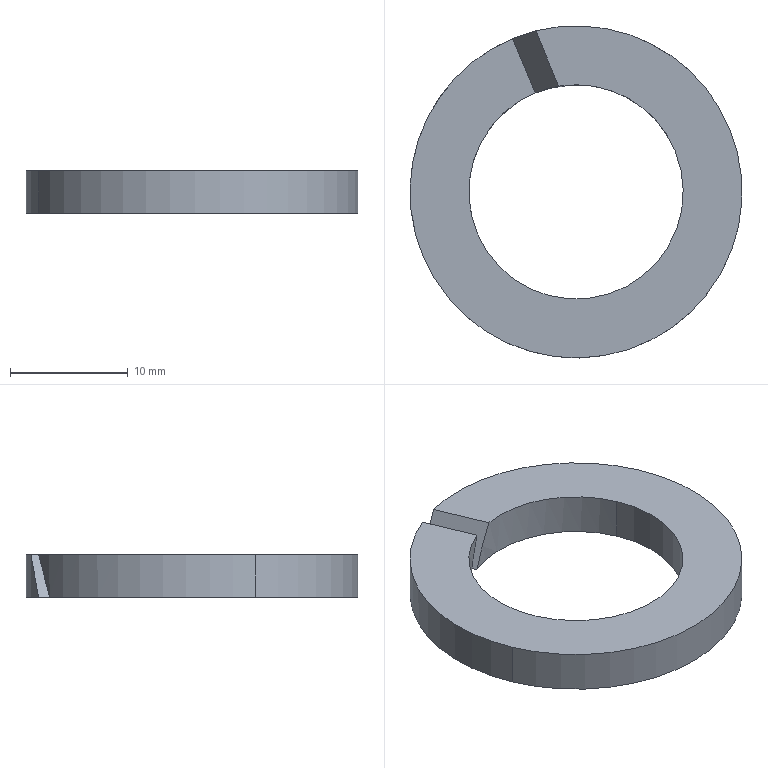Part | SolidWorks | features BaseBody 1 | 1 solid | 10 faces | box 28.2 x 28.2 x 3.6 mm | volume 1274 mm3 | cylinder 6 | plane 4 | commonest cylinder face diameters 18.2 x3 28.2 x3
STEP:
#1=CARTESIAN_POINT('',(-31.438,-44.703,125.25));
#2=VERTEX_POINT('',#1);
#3=CARTESIAN_POINT('',(-57.487,-55.505,125.25));
#4=VERTEX_POINT('',#3);
#5=CARTESIAN_POINT('',(-44.463,-50.104,125.25));
#6=DIRECTION('',(0.,0.,-1.));
#7=DIRECTION('',(-0.9237,-0.383,0.));
#8=AXIS2_PLACEMENT_3D('',#5,#6,#7);
#9=CIRCLE('',#8,14.1);
#10=EDGE_CURVE('',#2,#4,#9,.T.);
#11=ORIENTED_EDGE('',*,*,#10,.F.);
#12=CARTESIAN_POINT('',(-31.438,-44.703,128.85));
#13=VERTEX_POINT('',#12);
#14=CARTESIAN_POINT('',(-31.438,-44.703,125.25));
#15=DIRECTION('',(0.,0.,1.));
#16=VECTOR('',#15,1000.);
#17=LINE('',#14,#16);
#18=EDGE_CURVE('',#2,#13,#17,.T.);
#19=ORIENTED_EDGE('',*,*,#18,.T.);
#20=CARTESIAN_POINT('',(-57.487,-55.505,128.85));
#21=VERTEX_POINT('',#20);
#22=CARTESIAN_POINT('',(-44.463,-50.104,128.85));
#23=DIRECTION('',(0.,0.,-1.));
#24=DIRECTION('',(0.9237,0.383,0.));
#25=AXIS2_PLACEMENT_3D('',#22,#23,#24);
#26=CIRCLE('',#25,14.1);
#27=EDGE_CURVE('',#13,#21,#26,.T.);
#28=ORIENTED_EDGE('',*,*,#27,.T.);
#29=CARTESIAN_POINT('',(-57.487,-55.505,125.25));
#30=DIRECTION('',(0.,0.,1.));
#31=VECTOR('',#30,1000.);
#32=LINE('',#29,#31);
#33=EDGE_CURVE('',#4,#21,#32,.T.);
#34=ORIENTED_EDGE('',*,*,#33,.F.);
#35=EDGE_LOOP('',(#11,#19,#28,#34));
#36=FACE_OUTER_BOUND('',#35,.T.);
#37=CARTESIAN_POINT('',(-44.463,-50.104,125.25));
#38=DIRECTION('',(0.,0.,1.));
#39=DIRECTION('',(-0.9237,-0.383,0.));
#40=AXIS2_PLACEMENT_3D('',#37,#38,#39);
#41=CYLINDRICAL_SURFACE('',#40,14.1);
#42=ADVANCED_FACE('',(#36),#41,.T.);
#43=CARTESIAN_POINT('',(-51.725,-38.018,125.25));
#44=VERTEX_POINT('',#43);
#45=CARTESIAN_POINT('',(-44.463,-50.104,125.25));
#46=DIRECTION('',(0.,0.,-1.));
#47=DIRECTION('',(-0.9237,-0.383,0.));
#48=AXIS2_PLACEMENT_3D('',#45,#46,#47);
#49=CIRCLE('',#48,14.1);
#50=EDGE_CURVE('',#4,#44,#49,.T.);
#51=ORIENTED_EDGE('',*,*,#50,.F.);
#52=ORIENTED_EDGE('',*,*,#33,.T.);
#53=CARTESIAN_POINT('',(-49.864,-37.079,128.85));
#54=VERTEX_POINT('',#53);
#55=CARTESIAN_POINT('',(-44.463,-50.104,128.85));
#56=DIRECTION('',(0.,0.,-1.));
#57=DIRECTION('',(0.9237,0.383,0.));
#58=AXIS2_PLACEMENT_3D('',#55,#56,#57);
#59=CIRCLE('',#58,14.1);
#60=EDGE_CURVE('',#21,#54,#59,.T.);
#61=ORIENTED_EDGE('',*,*,#60,.T.);
#62=CARTESIAN_POINT('',(-51.725,-38.018,125.25));
#63=CARTESIAN_POINT('',(-51.128,-37.659,126.442));
#64=CARTESIAN_POINT('',(-50.507,-37.346,127.645));
#65=CARTESIAN_POINT('',(-49.864,-37.079,128.85));
#66=(BOUNDED_CURVE()B_SPLINE_CURVE(3,(#62,#63,#64,#65),.UNSPECIFIED.,.F.,.F.)B_SPLINE_CURVE_WITH_KNOTS((4,4),(4.564,4.712),.UNSPECIFIED.)CURVE()GEOMETRIC_REPRESENTATION_ITEM()RATIONAL_B_SPLINE_CURVE((1.,0.9982,0.9982,1.))REPRESENTATION_ITEM(''));
#67=EDGE_CURVE('',#44,#54,#66,.T.);
#68=ORIENTED_EDGE('',*,*,#67,.F.);
#69=EDGE_LOOP('',(#51,#52,#61,#68));
#70=FACE_OUTER_BOUND('',#69,.T.);
#71=CARTESIAN_POINT('',(-44.463,-50.104,125.25));
#72=DIRECTION('',(0.,0.,1.));
#73=DIRECTION('',(-0.9237,-0.383,0.));
#74=AXIS2_PLACEMENT_3D('',#71,#72,#73);
#75=CYLINDRICAL_SURFACE('',#74,14.1);
#76=ADVANCED_FACE('',(#70),#75,.T.);
#77=CARTESIAN_POINT('',(-47.949,-41.698,125.25));
#78=VERTEX_POINT('',#77);
#79=CARTESIAN_POINT('',(-36.057,-46.618,125.25));
#80=VERTEX_POINT('',#79);
#81=CARTESIAN_POINT('',(-44.463,-50.104,125.25));
#82=DIRECTION('',(0.,0.,-1.));
#83=DIRECTION('',(-0.9237,-0.383,0.));
#84=AXIS2_PLACEMENT_3D('',#81,#82,#83);
#85=CIRCLE('',#84,9.1);
#86=EDGE_CURVE('',#78,#80,#85,.T.);
#87=ORIENTED_EDGE('',*,*,#86,.T.);
#88=CARTESIAN_POINT('',(-36.057,-46.618,128.85));
#89=VERTEX_POINT('',#88);
#90=CARTESIAN_POINT('',(-36.057,-46.618,125.25));
#91=DIRECTION('',(0.,0.,1.));
#92=VECTOR('',#91,1000.);
#93=LINE('',#90,#92);
#94=EDGE_CURVE('',#80,#89,#93,.T.);
#95=ORIENTED_EDGE('',*,*,#94,.T.);
#96=CARTESIAN_POINT('',(-45.937,-41.124,128.85));
#97=VERTEX_POINT('',#96);
#98=CARTESIAN_POINT('',(-44.463,-50.104,128.85));
#99=DIRECTION('',(0.,0.,-1.));
#100=DIRECTION('',(0.9237,0.383,0.));
#101=AXIS2_PLACEMENT_3D('',#98,#99,#100);
#102=CIRCLE('',#101,9.1);
#103=EDGE_CURVE('',#97,#89,#102,.T.);
#104=ORIENTED_EDGE('',*,*,#103,.F.);
#105=CARTESIAN_POINT('',(-45.937,-41.124,128.85));
#106=CARTESIAN_POINT('',(-46.628,-41.237,127.669));
#107=CARTESIAN_POINT('',(-47.302,-41.43,126.463));
#108=CARTESIAN_POINT('',(-47.949,-41.698,125.25));
#109=(BOUNDED_CURVE()B_SPLINE_CURVE(3,(#105,#106,#107,#108),.UNSPECIFIED.,.F.,.T.)B_SPLINE_CURVE_WITH_KNOTS((4,4),(1.34,1.571),.UNSPECIFIED.)CURVE()GEOMETRIC_REPRESENTATION_ITEM()RATIONAL_B_SPLINE_CURVE((1.,0.9956,0.9956,1.))REPRESENTATION_ITEM(''));
#110=EDGE_CURVE('',#97,#78,#109,.T.);
#111=ORIENTED_EDGE('',*,*,#110,.T.);
#112=EDGE_LOOP('',(#87,#95,#104,#111));
#113=FACE_OUTER_BOUND('',#112,.T.);
#114=CARTESIAN_POINT('',(-44.463,-50.104,125.25));
#115=DIRECTION('',(0.,0.,1.));
#116=DIRECTION('',(-0.9237,-0.383,0.));
#117=AXIS2_PLACEMENT_3D('',#114,#115,#116);
#118=CYLINDRICAL_SURFACE('',#117,9.1);
#119=ADVANCED_FACE('',(#113),#118,.F.);
#120=ORIENTED_EDGE('',*,*,#94,.F.);
#121=CARTESIAN_POINT('',(-52.869,-53.59,125.25));
#122=VERTEX_POINT('',#121);
#123=CARTESIAN_POINT('',(-44.463,-50.104,125.25));
#124=DIRECTION('',(0.,0.,-1.));
#125=DIRECTION('',(-0.9237,-0.383,0.));
#126=AXIS2_PLACEMENT_3D('',#123,#124,#125);
#127=CIRCLE('',#126,9.1);
#128=EDGE_CURVE('',#80,#122,#127,.T.);
#129=ORIENTED_EDGE('',*,*,#128,.T.);
#130=CARTESIAN_POINT('',(-52.869,-53.59,128.85));
#131=VERTEX_POINT('',#130);
#132=CARTESIAN_POINT('',(-52.869,-53.59,125.25));
#133=DIRECTION('',(0.,0.,1.));
#134=VECTOR('',#133,1000.);
#135=LINE('',#132,#134);
#136=EDGE_CURVE('',#122,#131,#135,.T.);
#137=ORIENTED_EDGE('',*,*,#136,.T.);
#138=CARTESIAN_POINT('',(-44.463,-50.104,128.85));
#139=DIRECTION('',(0.,0.,-1.));
#140=DIRECTION('',(0.9237,0.383,0.));
#141=AXIS2_PLACEMENT_3D('',#138,#139,#140);
#142=CIRCLE('',#141,9.1);
#143=EDGE_CURVE('',#89,#131,#142,.T.);
#144=ORIENTED_EDGE('',*,*,#143,.F.);
#145=EDGE_LOOP('',(#120,#129,#137,#144));
#146=FACE_OUTER_BOUND('',#145,.T.);
#147=CARTESIAN_POINT('',(-44.463,-50.104,125.25));
#148=DIRECTION('',(0.,0.,1.));
#149=DIRECTION('',(-0.9237,-0.383,0.));
#150=AXIS2_PLACEMENT_3D('',#147,#148,#149);
#151=CYLINDRICAL_SURFACE('',#150,9.1);
#152=ADVANCED_FACE('',(#146),#151,.F.);
#153=CARTESIAN_POINT('',(-47.885,-36.425,128.85));
#154=VERTEX_POINT('',#153);
#155=CARTESIAN_POINT('',(-49.864,-37.079,125.25));
#156=VERTEX_POINT('',#155);
#157=CARTESIAN_POINT('',(-47.885,-36.425,128.85));
#158=CARTESIAN_POINT('',(-48.56,-36.594,127.658));
#159=CARTESIAN_POINT('',(-49.221,-36.813,126.455));
#160=CARTESIAN_POINT('',(-49.864,-37.079,125.25));
#161=(BOUNDED_CURVE()B_SPLINE_CURVE(3,(#157,#158,#159,#160),.UNSPECIFIED.,.F.,.F.)B_SPLINE_CURVE_WITH_KNOTS((4,4),(1.423,1.571),.UNSPECIFIED.)CURVE()GEOMETRIC_REPRESENTATION_ITEM()RATIONAL_B_SPLINE_CURVE((1.,0.9982,0.9982,1.))REPRESENTATION_ITEM(''));
#162=EDGE_CURVE('',#154,#156,#161,.T.);
#163=ORIENTED_EDGE('',*,*,#162,.T.);
#164=CARTESIAN_POINT('',(-49.864,-37.078,125.25));
#165=DIRECTION('',(0.383,-0.9237,0.));
#166=VECTOR('',#165,1000.);
#167=LINE('',#164,#166);
#168=EDGE_CURVE('',#156,#78,#167,.T.);
#169=ORIENTED_EDGE('',*,*,#168,.T.);
#170=ORIENTED_EDGE('',*,*,#110,.F.);
#171=CARTESIAN_POINT('',(-47.944,-36.282,128.85));
#172=DIRECTION('',(0.383,-0.9237,0.));
#173=VECTOR('',#172,1000.);
#174=LINE('',#171,#173);
#175=EDGE_CURVE('',#154,#97,#174,.T.);
#176=ORIENTED_EDGE('',*,*,#175,.F.);
#177=EDGE_LOOP('',(#163,#169,#170,#176));
#178=FACE_OUTER_BOUND('',#177,.T.);
#179=CARTESIAN_POINT('',(-47.944,-36.282,128.85));
#180=DIRECTION('',(0.8,0.3317,-0.5));
#181=DIRECTION('',(0.,-0.8333,-0.5528));
#182=AXIS2_PLACEMENT_3D('',#179,#180,#181);
#183=PLANE('',#182);
#184=ADVANCED_FACE('',(#178),#183,.F.);
#185=ORIENTED_EDGE('',*,*,#67,.T.);
#186=CARTESIAN_POINT('',(-47.949,-41.698,128.85));
#187=VERTEX_POINT('',#186);
#188=CARTESIAN_POINT('',(-49.864,-37.078,128.85));
#189=DIRECTION('',(0.383,-0.9237,0.));
#190=VECTOR('',#189,1000.);
#191=LINE('',#188,#190);
#192=EDGE_CURVE('',#54,#187,#191,.T.);
#193=ORIENTED_EDGE('',*,*,#192,.T.);
#194=CARTESIAN_POINT('',(-49.776,-42.716,125.25));
#195=VERTEX_POINT('',#194);
#196=CARTESIAN_POINT('',(-49.776,-42.716,125.25));
#197=CARTESIAN_POINT('',(-49.208,-42.307,126.431));
#198=CARTESIAN_POINT('',(-48.596,-41.966,127.637));
#199=CARTESIAN_POINT('',(-47.949,-41.698,128.85));
#200=(BOUNDED_CURVE()B_SPLINE_CURVE(3,(#196,#197,#198,#199),.UNSPECIFIED.,.F.,.F.)B_SPLINE_CURVE_WITH_KNOTS((4,4),(4.482,4.712),.UNSPECIFIED.)CURVE()GEOMETRIC_REPRESENTATION_ITEM()RATIONAL_B_SPLINE_CURVE((1.,0.9956,0.9956,1.))REPRESENTATION_ITEM(''));
#201=EDGE_CURVE('',#195,#187,#200,.T.);
#202=ORIENTED_EDGE('',*,*,#201,.F.);
#203=CARTESIAN_POINT('',(-51.784,-37.874,125.25));
#204=DIRECTION('',(0.383,-0.9237,0.));
#205=VECTOR('',#204,1000.);
#206=LINE('',#203,#205);
#207=EDGE_CURVE('',#44,#195,#206,.T.);
#208=ORIENTED_EDGE('',*,*,#207,.F.);
#209=EDGE_LOOP('',(#185,#193,#202,#208));
#210=FACE_OUTER_BOUND('',#209,.T.);
#211=CARTESIAN_POINT('',(-51.784,-37.874,125.25));
#212=DIRECTION('',(-0.8,-0.3317,0.5));
#213=DIRECTION('',(-0.383,0.9237,0.));
#214=AXIS2_PLACEMENT_3D('',#211,#212,#213);
#215=PLANE('',#214);
#216=ADVANCED_FACE('',(#210),#215,.F.);
#217=ORIENTED_EDGE('',*,*,#136,.F.);
#218=CARTESIAN_POINT('',(-44.463,-50.104,125.25));
#219=DIRECTION('',(0.,0.,-1.));
#220=DIRECTION('',(-0.9237,-0.383,0.));
#221=AXIS2_PLACEMENT_3D('',#218,#219,#220);
#222=CIRCLE('',#221,9.1);
#223=EDGE_CURVE('',#122,#195,#222,.T.);
#224=ORIENTED_EDGE('',*,*,#223,.T.);
#225=ORIENTED_EDGE('',*,*,#201,.T.);
#226=CARTESIAN_POINT('',(-44.463,-50.104,128.85));
#227=DIRECTION('',(0.,0.,-1.));
#228=DIRECTION('',(0.9237,0.383,0.));
#229=AXIS2_PLACEMENT_3D('',#226,#227,#228);
#230=CIRCLE('',#229,9.1);
#231=EDGE_CURVE('',#131,#187,#230,.T.);
#232=ORIENTED_EDGE('',*,*,#231,.F.);
#233=EDGE_LOOP('',(#217,#224,#225,#232));
#234=FACE_OUTER_BOUND('',#233,.T.);
#235=CARTESIAN_POINT('',(-44.463,-50.104,125.25));
#236=DIRECTION('',(0.,0.,1.));
#237=DIRECTION('',(-0.9237,-0.383,0.));
#238=AXIS2_PLACEMENT_3D('',#235,#236,#237);
#239=CYLINDRICAL_SURFACE('',#238,9.1);
#240=ADVANCED_FACE('',(#234),#239,.F.);
#241=ORIENTED_EDGE('',*,*,#18,.F.);
#242=CARTESIAN_POINT('',(-44.463,-50.104,125.25));
#243=DIRECTION('',(0.,0.,-1.));
#244=DIRECTION('',(-0.9237,-0.383,0.));
#245=AXIS2_PLACEMENT_3D('',#242,#243,#244);
#246=CIRCLE('',#245,14.1);
#247=EDGE_CURVE('',#156,#2,#246,.T.);
#248=ORIENTED_EDGE('',*,*,#247,.F.);
#249=ORIENTED_EDGE('',*,*,#162,.F.);
#250=CARTESIAN_POINT('',(-44.463,-50.104,128.85));
#251=DIRECTION('',(0.,0.,-1.));
#252=DIRECTION('',(0.9237,0.383,0.));
#253=AXIS2_PLACEMENT_3D('',#250,#251,#252);
#254=CIRCLE('',#253,14.1);
#255=EDGE_CURVE('',#154,#13,#254,.T.);
#256=ORIENTED_EDGE('',*,*,#255,.T.);
#257=EDGE_LOOP('',(#241,#248,#249,#256));
#258=FACE_OUTER_BOUND('',#257,.T.);
#259=CARTESIAN_POINT('',(-44.463,-50.104,125.25));
#260=DIRECTION('',(0.,0.,1.));
#261=DIRECTION('',(-0.9237,-0.383,0.));
#262=AXIS2_PLACEMENT_3D('',#259,#260,#261);
#263=CYLINDRICAL_SURFACE('',#262,14.1);
#264=ADVANCED_FACE('',(#258),#263,.T.);
#265=ORIENTED_EDGE('',*,*,#175,.T.);
#266=ORIENTED_EDGE('',*,*,#103,.T.);
#267=ORIENTED_EDGE('',*,*,#143,.T.);
#268=ORIENTED_EDGE('',*,*,#231,.T.);
#269=ORIENTED_EDGE('',*,*,#192,.F.);
#270=ORIENTED_EDGE('',*,*,#60,.F.);
#271=ORIENTED_EDGE('',*,*,#27,.F.);
#272=ORIENTED_EDGE('',*,*,#255,.F.);
#273=EDGE_LOOP('',(#265,#266,#267,#268,#269,#270,#271,#272));
#274=FACE_OUTER_BOUND('',#273,.T.);
#275=CARTESIAN_POINT('',(-44.463,-50.104,128.85));
#276=DIRECTION('',(0.,0.,1.));
#277=DIRECTION('',(0.,-1.,0.));
#278=AXIS2_PLACEMENT_3D('',#275,#276,#277);
#279=PLANE('',#278);
#280=ADVANCED_FACE('',(#274),#279,.T.);
#281=ORIENTED_EDGE('',*,*,#86,.F.);
#282=ORIENTED_EDGE('',*,*,#168,.F.);
#283=ORIENTED_EDGE('',*,*,#247,.T.);
#284=ORIENTED_EDGE('',*,*,#10,.T.);
#285=ORIENTED_EDGE('',*,*,#50,.T.);
#286=ORIENTED_EDGE('',*,*,#207,.T.);
#287=ORIENTED_EDGE('',*,*,#223,.F.);
#288=ORIENTED_EDGE('',*,*,#128,.F.);
#289=EDGE_LOOP('',(#281,#282,#283,#284,#285,#286,#287,#288));
#290=FACE_OUTER_BOUND('',#289,.T.);
#291=CARTESIAN_POINT('',(-44.463,-50.104,125.25));
#292=DIRECTION('',(0.,0.,1.));
#293=DIRECTION('',(0.,-1.,0.));
#294=AXIS2_PLACEMENT_3D('',#291,#292,#293);
#295=PLANE('',#294);
#296=ADVANCED_FACE('',(#290),#295,.F.);
#297=CLOSED_SHELL('',(#42,#76,#119,#152,#184,#216,#240,#264,#280,#296));
#298=MANIFOLD_SOLID_BREP('',#297);
#299=CARTESIAN_POINT('',(0.,0.,0.));
#300=DIRECTION('',(0.,0.,1.));
#301=DIRECTION('',(1.,0.,0.));
#302=AXIS2_PLACEMENT_3D('',#299,#300,#301);
#303=(LENGTH_UNIT()NAMED_UNIT(*)SI_UNIT(.MILLI.,.METRE.));
#304=UNCERTAINTY_MEASURE_WITH_UNIT(LENGTH_MEASURE(0.00001),#303,'','');
#305=(NAMED_UNIT(*)PLANE_ANGLE_UNIT()SI_UNIT($,.RADIAN.));
#306=(NAMED_UNIT(*)SI_UNIT($,.STERADIAN.)SOLID_ANGLE_UNIT());
#307=(GEOMETRIC_REPRESENTATION_CONTEXT(3)GLOBAL_UNCERTAINTY_ASSIGNED_CONTEXT((#304))GLOBAL_UNIT_ASSIGNED_CONTEXT((#303,#305,#306))REPRESENTATION_CONTEXT('',''));
#308=ADVANCED_BREP_SHAPE_REPRESENTATION('',(#298,#302),#307);